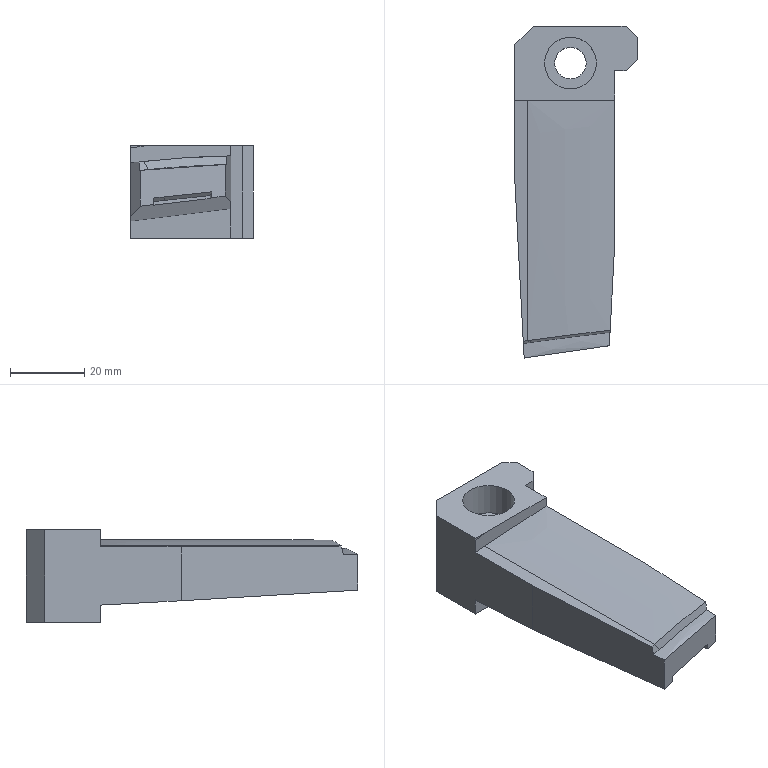Part | STEP file | P011002S001-002 | 1 solid | 30 faces | box 33 x 89.557 x 25 mm | volume 35725 mm3 | plane 18 | spline 7 | other 3 | cylinder 2 | commonest cylinder face diameters 8.5 x1 14 x1